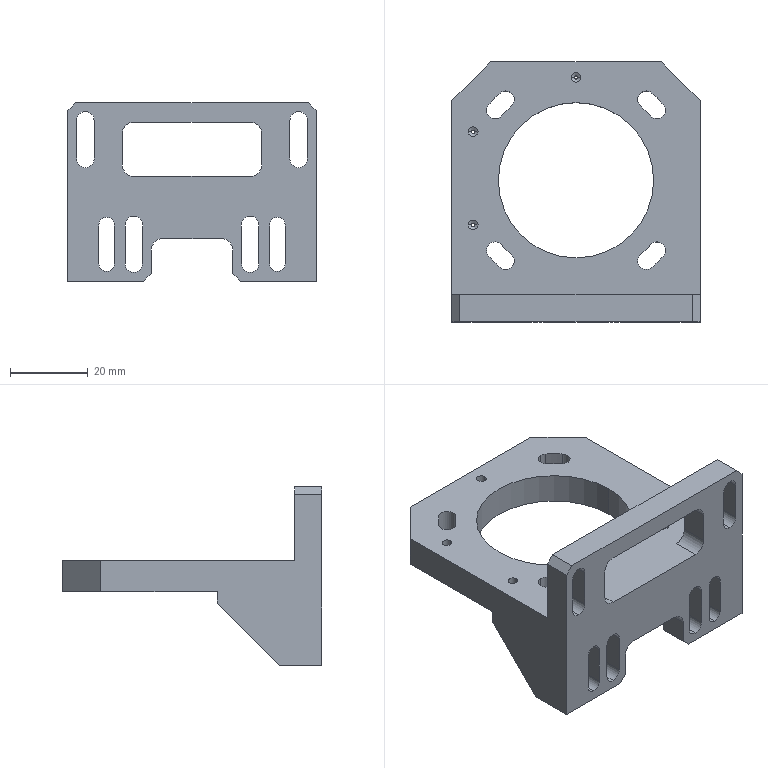NC program | NX | posted with a generic post | part box 64 x 67 x 46 mm
Lines 1 to 1063 of 33790:
N10 G17 G21 G94 G90
(ZLEVEL_PROFILE , TOOL : D10C)
N12 T10 M6
N14 G54
N16 G17 G0 G90 X-38.6 Y9.489 B0. C0. S2500 M3
N18 G43 Z30. H10
N20 Z1.5
N22 G94 G1 Y32.32 Z0.303 F1000.
N24 X-38.483 Y33.131 Z0.261
N26 X-38.238 Y33.914 Z0.218
N28 X-37.871 Y34.647 Z0.175
N30 X-37.392 Y35.312 Z0.132
N32 X-36.812 Y35.892 Z0.089
N34 X-36.147 Y36.371 Z0.046
N36 X-35.414 Y36.738 Z0.003
N38 X-34.631 Y36.983 Z-0.04
N40 X-33.82 Y37.1 Z-0.083
N42 X-33.5 Z-0.1
N44 X23.5 F2500.
N46 G2 X27.106 Y35.606 R5.1
N48 G1 X37.106 Y25.606
N50 G2 X38.6 Y22. R5.1
N52 G1 Y-22.
N54 G2 X37.106 Y-25.606 R5.1
N56 G1 X27.106 Y-35.606
N58 G2 X23.5 Y-37.1 R5.1
N60 G1 X-33.5
N62 G2 X-38.6 Y-32. R5.1
N64 G1 Y32.
N66 G2 X-33.5 Y37.1 R5.1
N68 G1 X-27.771 Z-0.2
N70 X23.5
N72 G2 X27.106 Y35.606 R5.1
N74 G1 X37.106 Y25.606
N76 G2 X38.6 Y22. R5.1
N78 G1 Y-22.
N80 G2 X37.106 Y-25.606 R5.1
N82 G1 X27.106 Y-35.606
N84 G2 X23.5 Y-37.1 R5.1
N86 G1 X-33.5
N88 G2 X-38.6 Y-32. R5.1
N90 G1 Y32.
N92 G2 X-33.5 Y37.1 R5.1
N94 G1 X-27.771 Z-0.3
N96 X23.5
N98 G2 X27.106 Y35.606 R5.1
N100 G1 X37.106 Y25.606
N102 G2 X38.6 Y22. R5.1
N104 G1 Y-22.
N106 G2 X37.106 Y-25.606 R5.1
N108 G1 X27.106 Y-35.606
N110 G2 X23.5 Y-37.1 R5.1
N112 G1 X-33.5
N114 G2 X-38.6 Y-32. R5.1
N116 G1 Y32.
N118 G2 X-33.5 Y37.1 R5.1
N120 G1 X-27.771 Z-0.4
N122 X23.5
N124 G2 X27.106 Y35.606 R5.1
N126 G1 X37.106 Y25.606
N128 G2 X38.6 Y22. R5.1
N130 G1 Y-22.
N132 G2 X37.106 Y-25.606 R5.1
N134 G1 X27.106 Y-35.606
N136 G2 X23.5 Y-37.1 R5.1
N138 G1 X-33.5
N140 G2 X-38.6 Y-32. R5.1
N142 G1 Y32.
N144 G2 X-33.5 Y37.1 R5.1
N146 G1 X-27.771 Z-0.5
N148 X23.5
N150 G2 X27.106 Y35.606 R5.1
N152 G1 X37.106 Y25.606
N154 G2 X38.6 Y22. R5.1
N156 G1 Y-22.
N158 G2 X37.106 Y-25.606 R5.1
N160 G1 X27.106 Y-35.606
N162 G2 X23.5 Y-37.1 R5.1
N164 G1 X-33.5
N166 G2 X-38.6 Y-32. R5.1
N168 G1 Y32.
N170 G2 X-33.5 Y37.1 R5.1
N172 G1 X-27.771 Z-0.6
N174 X23.5
N176 G2 X27.106 Y35.606 R5.1
N178 G1 X37.106 Y25.606
N180 G2 X38.6 Y22. R5.1
N182 G1 Y-22.
N184 G2 X37.106 Y-25.606 R5.1
N186 G1 X27.106 Y-35.606
N188 G2 X23.5 Y-37.1 R5.1
N190 G1 X-33.5
N192 G2 X-38.6 Y-32. R5.1
N194 G1 Y32.
N196 G2 X-33.5 Y37.1 R5.1
N198 G1 X-27.771 Z-0.7
N200 X23.5
N202 G2 X27.106 Y35.606 R5.1
N204 G1 X37.106 Y25.606
N206 G2 X38.6 Y22. R5.1
N208 G1 Y-22.
N210 G2 X37.106 Y-25.606 R5.1
N212 G1 X27.106 Y-35.606
N214 G2 X23.5 Y-37.1 R5.1
N216 G1 X-33.5
N218 G2 X-38.6 Y-32. R5.1
N220 G1 Y32.
N222 G2 X-33.5 Y37.1 R5.1
N224 G1 X-27.771 Z-0.8
N226 X23.5
N228 G2 X27.106 Y35.606 R5.1
N230 G1 X37.106 Y25.606
N232 G2 X38.6 Y22. R5.1
N234 G1 Y-22.
N236 G2 X37.106 Y-25.606 R5.1
N238 G1 X27.106 Y-35.606
N240 G2 X23.5 Y-37.1 R5.1
N242 G1 X-33.5
N244 G2 X-38.6 Y-32. R5.1
N246 G1 Y32.
N248 G2 X-33.5 Y37.1 R5.1
N250 G1 X-27.771 Z-0.9
N252 X23.5
N254 G2 X27.106 Y35.606 R5.1
N256 G1 X37.106 Y25.606
N258 G2 X38.6 Y22. R5.1
N260 G1 Y-22.
N262 G2 X37.106 Y-25.606 R5.1
N264 G1 X27.106 Y-35.606
N266 G2 X23.5 Y-37.1 R5.1
N268 G1 X-33.5
N270 G2 X-38.6 Y-32. R5.1
N272 G1 Y32.
N274 G2 X-33.5 Y37.1 R5.1
N276 G1 X-27.771 Z-1.
N278 X23.5
N280 G2 X27.106 Y35.606 R5.1
N282 G1 X37.106 Y25.606
N284 G2 X38.6 Y22. R5.1
N286 G1 Y-22.
N288 G2 X37.106 Y-25.606 R5.1
N290 G1 X27.106 Y-35.606
N292 G2 X23.5 Y-37.1 R5.1
N294 G1 X-33.5
N296 G2 X-38.6 Y-32. R5.1
N298 G1 Y32.
N300 G2 X-33.5 Y37.1 R5.1
N302 G1 X-27.771 Z-1.1
N304 X23.5
N306 G2 X27.106 Y35.606 R5.1
N308 G1 X37.106 Y25.606
N310 G2 X38.6 Y22. R5.1
N312 G1 Y-22.
N314 G2 X37.106 Y-25.606 R5.1
N316 G1 X27.106 Y-35.606
N318 G2 X23.5 Y-37.1 R5.1
N320 G1 X-33.5
N322 G2 X-38.6 Y-32. R5.1
N324 G1 Y32.
N326 G2 X-33.5 Y37.1 R5.1
N328 G1 X-27.771 Z-1.2
N330 X23.5
N332 G2 X27.106 Y35.606 R5.1
N334 G1 X37.106 Y25.606
N336 G2 X38.6 Y22. R5.1
N338 G1 Y-22.
N340 G2 X37.106 Y-25.606 R5.1
N342 G1 X27.106 Y-35.606
N344 G2 X23.5 Y-37.1 R5.1
N346 G1 X-33.5
N348 G2 X-38.6 Y-32. R5.1
N350 G1 Y32.
N352 G2 X-33.5 Y37.1 R5.1
N354 G1 X-27.771 Z-1.3
N356 X23.5
N358 G2 X27.106 Y35.606 R5.1
N360 G1 X37.106 Y25.606
N362 G2 X38.6 Y22. R5.1
N364 G1 Y-22.
N366 G2 X37.106 Y-25.606 R5.1
N368 G1 X27.106 Y-35.606
N370 G2 X23.5 Y-37.1 R5.1
N372 G1 X-33.5
N374 G2 X-38.6 Y-32. R5.1
N376 G1 Y32.
N378 G2 X-33.5 Y37.1 R5.1
N380 G1 X-27.771 Z-1.4
N382 X23.5
N384 G2 X27.106 Y35.606 R5.1
N386 G1 X37.106 Y25.606
N388 G2 X38.6 Y22. R5.1
N390 G1 Y-22.
N392 G2 X37.106 Y-25.606 R5.1
N394 G1 X27.106 Y-35.606
N396 G2 X23.5 Y-37.1 R5.1
N398 G1 X-33.5
N400 G2 X-38.6 Y-32. R5.1
N402 G1 Y32.
N404 G2 X-33.5 Y37.1 R5.1
N406 G1 X-27.771 Z-1.5
N408 X23.5
N410 G2 X27.106 Y35.606 R5.1
N412 G1 X37.106 Y25.606
N414 G2 X38.6 Y22. R5.1
N416 G1 Y-22.
N418 G2 X37.106 Y-25.606 R5.1
N420 G1 X27.106 Y-35.606
N422 G2 X23.5 Y-37.1 R5.1
N424 G1 X-33.5
N426 G2 X-38.6 Y-32. R5.1
N428 G1 Y32.
N430 G2 X-33.5 Y37.1 R5.1
N432 G1 X-27.771 Z-1.6
N434 X23.5
N436 G2 X27.106 Y35.606 R5.1
N438 G1 X37.106 Y25.606
N440 G2 X38.6 Y22. R5.1
N442 G1 Y-22.
N444 G2 X37.106 Y-25.606 R5.1
N446 G1 X27.106 Y-35.606
N448 G2 X23.5 Y-37.1 R5.1
N450 G1 X-33.5
N452 G2 X-38.6 Y-32. R5.1
N454 G1 Y32.
N456 G2 X-33.5 Y37.1 R5.1
N458 G1 X-27.771 Z-1.7
N460 X23.5
N462 G2 X27.106 Y35.606 R5.1
N464 G1 X37.106 Y25.606
N466 G2 X38.6 Y22. R5.1
N468 G1 Y-22.
N470 G2 X37.106 Y-25.606 R5.1
N472 G1 X27.106 Y-35.606
N474 G2 X23.5 Y-37.1 R5.1
N476 G1 X-33.5
N478 G2 X-38.6 Y-32. R5.1
N480 G1 Y32.
N482 G2 X-33.5 Y37.1 R5.1
N484 G1 X-27.771 Z-1.8
N486 X23.5
N488 G2 X27.106 Y35.606 R5.1
N490 G1 X37.106 Y25.606
N492 G2 X38.6 Y22. R5.1
N494 G1 Y-22.
N496 G2 X37.106 Y-25.606 R5.1
N498 G1 X27.106 Y-35.606
N500 G2 X23.5 Y-37.1 R5.1
N502 G1 X-33.5
N504 G2 X-38.6 Y-32. R5.1
N506 G1 Y32.
N508 G2 X-33.5 Y37.1 R5.1
N510 G1 X-27.771 Z-1.9
N512 X23.5
N514 G2 X27.106 Y35.606 R5.1
N516 G1 X37.106 Y25.606
N518 G2 X38.6 Y22. R5.1
N520 G1 Y-22.
N522 G2 X37.106 Y-25.606 R5.1
N524 G1 X27.106 Y-35.606
N526 G2 X23.5 Y-37.1 R5.1
N528 G1 X-33.5
N530 G2 X-38.6 Y-32. R5.1
N532 G1 Y32.
N534 G2 X-33.5 Y37.1 R5.1
N536 G1 X-27.771 Z-2.
N538 X23.5
N540 G2 X27.106 Y35.606 R5.1
N542 G1 X37.106 Y25.606
N544 G2 X38.6 Y22. R5.1
N546 G1 Y-22.
N548 G2 X37.106 Y-25.606 R5.1
N550 G1 X27.106 Y-35.606
N552 G2 X23.5 Y-37.1 R5.1
N554 G1 X-33.5
N556 G2 X-38.6 Y-32. R5.1
N558 G1 Y32.
N560 G2 X-33.5 Y37.1 R5.1
N562 G1 X-27.771 Z-2.1
N564 X23.5
N566 G2 X27.106 Y35.606 R5.1
N568 G1 X37.106 Y25.606
N570 G2 X38.6 Y22. R5.1
N572 G1 Y-22.
N574 G2 X37.106 Y-25.606 R5.1
N576 G1 X27.106 Y-35.606
N578 G2 X23.5 Y-37.1 R5.1
N580 G1 X-33.5
N582 G2 X-38.6 Y-32. R5.1
N584 G1 Y32.
N586 G2 X-33.5 Y37.1 R5.1
N588 G1 X-27.771 Z-2.2
N590 X23.5
N592 G2 X27.106 Y35.606 R5.1
N594 G1 X37.106 Y25.606
N596 G2 X38.6 Y22. R5.1
N598 G1 Y-22.
N600 G2 X37.106 Y-25.606 R5.1
N602 G1 X27.106 Y-35.606
N604 G2 X23.5 Y-37.1 R5.1
N606 G1 X-33.5
N608 G2 X-38.6 Y-32. R5.1
N610 G1 Y32.
N612 G2 X-33.5 Y37.1 R5.1
N614 G1 X-27.771 Z-2.3
N616 X23.5
N618 G2 X27.106 Y35.606 R5.1
N620 G1 X37.106 Y25.606
N622 G2 X38.6 Y22. R5.1
N624 G1 Y-22.
N626 G2 X37.106 Y-25.606 R5.1
N628 G1 X27.106 Y-35.606
N630 G2 X23.5 Y-37.1 R5.1
N632 G1 X-33.5
N634 G2 X-38.6 Y-32. R5.1
N636 G1 Y32.
N638 G2 X-33.5 Y37.1 R5.1
N640 G1 X-27.771 Z-2.4
N642 X23.5
N644 G2 X27.106 Y35.606 R5.1
N646 G1 X37.106 Y25.606
N648 G2 X38.6 Y22. R5.1
N650 G1 Y-22.
N652 G2 X37.106 Y-25.606 R5.1
N654 G1 X27.106 Y-35.606
N656 G2 X23.5 Y-37.1 R5.1
N658 G1 X-33.5
N660 G2 X-38.6 Y-32. R5.1
N662 G1 Y32.
N664 G2 X-33.5 Y37.1 R5.1
N666 G1 X-27.771 Z-2.5
N668 X23.5
N670 G2 X27.106 Y35.606 R5.1
N672 G1 X37.106 Y25.606
N674 G2 X38.6 Y22. R5.1
N676 G1 Y-22.
N678 G2 X37.106 Y-25.606 R5.1
N680 G1 X27.106 Y-35.606
N682 G2 X23.5 Y-37.1 R5.1
N684 G1 X-33.5
N686 G2 X-38.6 Y-32. R5.1
N688 G1 Y32.
N690 G2 X-33.5 Y37.1 R5.1
N692 G1 X-27.771 Z-2.6
N694 X23.5
N696 G2 X27.106 Y35.606 R5.1
N698 G1 X37.106 Y25.606
N700 G2 X38.6 Y22. R5.1
N702 G1 Y-22.
N704 G2 X37.106 Y-25.606 R5.1
N706 G1 X27.106 Y-35.606
N708 G2 X23.5 Y-37.1 R5.1
N710 G1 X-33.5
N712 G2 X-38.6 Y-32. R5.1
N714 G1 Y32.
N716 G2 X-33.5 Y37.1 R5.1
N718 G1 X-27.771 Z-2.7
N720 X23.5
N722 G2 X27.106 Y35.606 R5.1
N724 G1 X37.106 Y25.606
N726 G2 X38.6 Y22. R5.1
N728 G1 Y-22.
N730 G2 X37.106 Y-25.606 R5.1
N732 G1 X27.106 Y-35.606
N734 G2 X23.5 Y-37.1 R5.1
N736 G1 X-33.5
N738 G2 X-38.6 Y-32. R5.1
N740 G1 Y32.
N742 G2 X-33.5 Y37.1 R5.1
N744 G1 X-27.771 Z-2.8
N746 X23.5
N748 G2 X27.106 Y35.606 R5.1
N750 G1 X37.106 Y25.606
N752 G2 X38.6 Y22. R5.1
N754 G1 Y-22.
N756 G2 X37.106 Y-25.606 R5.1
N758 G1 X27.106 Y-35.606
N760 G2 X23.5 Y-37.1 R5.1
N762 G1 X-33.5
N764 G2 X-38.6 Y-32. R5.1
N766 G1 Y32.
N768 G2 X-33.5 Y37.1 R5.1
N770 G1 X-27.771 Z-2.9
N772 X23.5
N774 G2 X27.106 Y35.606 R5.1
N776 G1 X37.106 Y25.606
N778 G2 X38.6 Y22. R5.1
N780 G1 Y-22.
N782 G2 X37.106 Y-25.606 R5.1
N784 G1 X27.106 Y-35.606
N786 G2 X23.5 Y-37.1 R5.1
N788 G1 X-33.5
N790 G2 X-38.6 Y-32. R5.1
N792 G1 Y32.
N794 G2 X-33.5 Y37.1 R5.1
N796 G1 X-27.771 Z-3.
N798 X23.5
N800 G2 X27.106 Y35.606 R5.1
N802 G1 X37.106 Y25.606
N804 G2 X38.6 Y22. R5.1
N806 G1 Y-22.
N808 G2 X37.106 Y-25.606 R5.1
N810 G1 X27.106 Y-35.606
N812 G2 X23.5 Y-37.1 R5.1
N814 G1 X-33.5
N816 G2 X-38.6 Y-32. R5.1
N818 G1 Y32.
N820 G2 X-33.5 Y37.1 R5.1
N822 G1 X-27.771 Z-3.1
N824 X23.5
N826 G2 X27.106 Y35.606 R5.1
N828 G1 X37.106 Y25.606
N830 G2 X38.6 Y22. R5.1
N832 G1 Y-22.
N834 G2 X37.106 Y-25.606 R5.1
N836 G1 X27.106 Y-35.606
N838 G2 X23.5 Y-37.1 R5.1
N840 G1 X-33.5
N842 G2 X-38.6 Y-32. R5.1
N844 G1 Y32.
N846 G2 X-33.5 Y37.1 R5.1
N848 G1 X-27.771 Z-3.2
N850 X23.5
N852 G2 X27.106 Y35.606 R5.1
N854 G1 X37.106 Y25.606
N856 G2 X38.6 Y22. R5.1
N858 G1 Y-22.
N860 G2 X37.106 Y-25.606 R5.1
N862 G1 X27.106 Y-35.606
N864 G2 X23.5 Y-37.1 R5.1
N866 G1 X-33.5
N868 G2 X-38.6 Y-32. R5.1
N870 G1 Y32.
N872 G2 X-33.5 Y37.1 R5.1
N874 G1 X-27.771 Z-3.3
N876 X23.5
N878 G2 X27.106 Y35.606 R5.1
N880 G1 X37.106 Y25.606
N882 G2 X38.6 Y22. R5.1
N884 G1 Y-22.
N886 G2 X37.106 Y-25.606 R5.1
N888 G1 X27.106 Y-35.606
N890 G2 X23.5 Y-37.1 R5.1
N892 G1 X-33.5
N894 G2 X-38.6 Y-32. R5.1
N896 G1 Y32.
N898 G2 X-33.5 Y37.1 R5.1
N900 G1 X-27.771 Z-3.4
N902 X23.5
N904 G2 X27.106 Y35.606 R5.1
N906 G1 X37.106 Y25.606
N908 G2 X38.6 Y22. R5.1
N910 G1 Y-22.
N912 G2 X37.106 Y-25.606 R5.1
N914 G1 X27.106 Y-35.606
N916 G2 X23.5 Y-37.1 R5.1
N918 G1 X-33.5
N920 G2 X-38.6 Y-32. R5.1
N922 G1 Y32.
N924 G2 X-33.5 Y37.1 R5.1
N926 G1 X-27.771 Z-3.5
N928 X23.5
N930 G2 X27.106 Y35.606 R5.1
N932 G1 X37.106 Y25.606
N934 G2 X38.6 Y22. R5.1
N936 G1 Y-22.
N938 G2 X37.106 Y-25.606 R5.1
N940 G1 X27.106 Y-35.606
N942 G2 X23.5 Y-37.1 R5.1
N944 G1 X-33.5
N946 G2 X-38.6 Y-32. R5.1
N948 G1 Y32.
N950 G2 X-33.5 Y37.1 R5.1
N952 G1 X-27.771 Z-3.6
N954 X23.5
N956 G2 X27.106 Y35.606 R5.1
N958 G1 X37.106 Y25.606
N960 G2 X38.6 Y22. R5.1
N962 G1 Y-22.
N964 G2 X37.106 Y-25.606 R5.1
N966 G1 X27.106 Y-35.606
N968 G2 X23.5 Y-37.1 R5.1
N970 G1 X-33.5
N972 G2 X-38.6 Y-32. R5.1
N974 G1 Y32.
N976 G2 X-33.5 Y37.1 R5.1
N978 G1 X-27.771 Z-3.7
N980 X23.5
N982 G2 X27.106 Y35.606 R5.1
N984 G1 X37.106 Y25.606
N986 G2 X38.6 Y22. R5.1
N988 G1 Y-22.
N990 G2 X37.106 Y-25.606 R5.1
N992 G1 X27.106 Y-35.606
N994 G2 X23.5 Y-37.1 R5.1
N996 G1 X-33.5
N998 G2 X-38.6 Y-32. R5.1
N1000 G1 Y32.
N1002 G2 X-33.5 Y37.1 R5.1
N1004 G1 X-27.771 Z-3.8
N1006 X23.5
N1008 G2 X27.106 Y35.606 R5.1
N1010 G1 X37.106 Y25.606
N1012 G2 X38.6 Y22. R5.1
N1014 G1 Y-22.
N1016 G2 X37.106 Y-25.606 R5.1
N1018 G1 X27.106 Y-35.606
N1020 G2 X23.5 Y-37.1 R5.1
N1022 G1 X-33.5
N1024 G2 X-38.6 Y-32. R5.1
N1026 G1 Y32.
N1028 G2 X-33.5 Y37.1 R5.1
N1030 G1 X-27.771 Z-3.9
N1032 X23.5
N1034 G2 X27.106 Y35.606 R5.1
N1036 G1 X37.106 Y25.606
N1038 G2 X38.6 Y22. R5.1
N1040 G1 Y-22.
N1042 G2 X37.106 Y-25.606 R5.1
N1044 G1 X27.106 Y-35.606
N1046 G2 X23.5 Y-37.1 R5.1
N1048 G1 X-33.5
N1050 G2 X-38.6 Y-32. R5.1
N1052 G1 Y32.
N1054 G2 X-33.5 Y37.1 R5.1
N1056 G1 X-27.771 Z-4.
N1058 X23.5
N1060 G2 X27.106 Y35.606 R5.1
N1062 G1 X37.106 Y25.606
N1064 G2 X38.6 Y22. R5.1
N1066 G1 Y-22.
N1068 G2 X37.106 Y-25.606 R5.1
N1070 G1 X27.106 Y-35.606
N1072 G2 X23.5 Y-37.1 R5.1
N1074 G1 X-33.5
N1076 G2 X-38.6 Y-32. R5.1
N1078 G1 Y32.
N1080 G2 X-33.5 Y37.1 R5.1
N1082 G1 X-27.771 Z-4.1
N1084 X23.5
N1086 G2 X27.106 Y35.606 R5.1
N1088 G1 X37.106 Y25.606
N1090 G2 X38.6 Y22. R5.1
N1092 G1 Y-22.
N1094 G2 X37.106 Y-25.606 R5.1
N1096 G1 X27.106 Y-35.606
N1098 G2 X23.5 Y-37.1 R5.1
N1100 G1 X-33.5
N1102 G2 X-38.6 Y-32. R5.1
N1104 G1 Y32.
N1106 G2 X-33.5 Y37.1 R5.1
N1108 G1 X-27.771 Z-4.2
N1110 X23.5
N1112 G2 X27.106 Y35.606 R5.1
N1114 G1 X37.106 Y25.606
N1116 G2 X38.6 Y22. R5.1
N1118 G1 Y-22.
N1120 G2 X37.106 Y-25.606 R5.1
N1122 G1 X27.106 Y-35.606
N1124 G2 X23.5 Y-37.1 R5.1
N1126 G1 X-33.5
N1128 G2 X-38.6 Y-32. R5.1
N1130 G1 Y32.
N1132 G2 X-33.5 Y37.1 R5.1
N1134 G1 X-27.771 Z-4.3
N1136 X23.5
N1138 G2 X27.106 Y35.606 R5.1
N1140 G1 X37.106 Y25.606
N1142 G2 X38.6 Y22. R5.1
N1144 G1 Y-22.
N1146 G2 X37.106 Y-25.606 R5.1
N1148 G1 X27.106 Y-35.606
N1150 G2 X23.5 Y-37.1 R5.1
N1152 G1 X-33.5
N1154 G2 X-38.6 Y-32. R5.1
N1156 G1 Y32.
N1158 G2 X-33.5 Y37.1 R5.1
N1160 G1 X-27.771 Z-4.4
N1162 X23.5
N1164 G2 X27.106 Y35.606 R5.1
N1166 G1 X37.106 Y25.606
N1168 G2 X38.6 Y22. R5.1
N1170 G1 Y-22.
N1172 G2 X37.106 Y-25.606 R5.1
N1174 G1 X27.106 Y-35.606
N1176 G2 X23.5 Y-37.1 R5.1
N1178 G1 X-33.5
N1180 G2 X-38.6 Y-32. R5.1
N1182 G1 Y32.
N1184 G2 X-33.5 Y37.1 R5.1
N1186 G1 X-27.771 Z-4.5
N1188 X23.5
N1190 G2 X27.106 Y35.606 R5.1
N1192 G1 X37.106 Y25.606
N1194 G2 X38.6 Y22. R5.1
N1196 G1 Y-22.
N1198 G2 X37.106 Y-25.606 R5.1
N1200 G1 X27.106 Y-35.606
N1202 G2 X23.5 Y-37.1 R5.1
N1204 G1 X-33.5
N1206 G2 X-38.6 Y-32. R5.1
N1208 G1 Y32.
N1210 G2 X-33.5 Y37.1 R5.1
N1212 G1 X-27.771 Z-4.6
N1214 X23.5
N1216 G2 X27.106 Y35.606 R5.1
N1218 G1 X37.106 Y25.606
N1220 G2 X38.6 Y22. R5.1
N1222 G1 Y-22.
N1224 G2 X37.106 Y-25.606 R5.1
N1226 G1 X27.106 Y-35.606
N1228 G2 X23.5 Y-37.1 R5.1
N1230 G1 X-33.5
N1232 G2 X-38.6 Y-32. R5.1
N1234 G1 Y32.
N1236 G2 X-33.5 Y37.1 R5.1
N1238 G1 X-27.771 Z-4.7
N1240 X23.5
N1242 G2 X27.106 Y35.606 R5.1
N1244 G1 X37.106 Y25.606
N1246 G2 X38.6 Y22. R5.1
N1248 G1 Y-22.
N1250 G2 X37.106 Y-25.606 R5.1
N1252 G1 X27.106 Y-35.606
N1254 G2 X23.5 Y-37.1 R5.1
N1256 G1 X-33.5
N1258 G2 X-38.6 Y-32. R5.1
N1260 G1 Y32.
N1262 G2 X-33.5 Y37.1 R5.1
N1264 G1 X-27.771 Z-4.8
N1266 X23.5
N1268 G2 X27.106 Y35.606 R5.1
N1270 G1 X37.106 Y25.606
N1272 G2 X38.6 Y22. R5.1
N1274 G1 Y-22.
N1276 G2 X37.106 Y-25.606 R5.1
N1278 G1 X27.106 Y-35.606
N1280 G2 X23.5 Y-37.1 R5.1
N1282 G1 X-33.5
N1284 G2 X-38.6 Y-32. R5.1
N1286 G1 Y32.
N1288 G2 X-33.5 Y37.1 R5.1
N1290 G1 X-27.771 Z-4.9
N1292 X23.5
N1294 G2 X27.106 Y35.606 R5.1
N1296 G1 X37.106 Y25.606
N1298 G2 X38.6 Y22. R5.1
N1300 G1 Y-22.
N1302 G2 X37.106 Y-25.606 R5.1
N1304 G1 X27.106 Y-35.606
N1306 G2 X23.5 Y-37.1 R5.1
N1308 G1 X-33.5
N1310 G2 X-38.6 Y-32. R5.1
N1312 G1 Y32.
N1314 G2 X-33.5 Y37.1 R5.1
N1316 G1 X-27.771 Z-5.
N1318 X23.5
N1320 G2 X27.106 Y35.606 R5.1
N1322 G1 X37.106 Y25.606
N1324 G2 X38.6 Y22. R5.1
N1326 G1 Y-22.
N1328 G2 X37.106 Y-25.606 R5.1
N1330 G1 X27.106 Y-35.606
N1332 G2 X23.5 Y-37.1 R5.1
N1334 G1 X-33.5
N1336 G2 X-38.6 Y-32. R5.1
N1338 G1 Y32.
N1340 G2 X-33.5 Y37.1 R5.1
N1342 G1 X-27.771 Z-5.1
N1344 X23.5
N1346 G2 X27.106 Y35.606 R5.1
N1348 G1 X37.106 Y25.606
N1350 G2 X38.6 Y22. R5.1
N1352 G1 Y-22.
N1354 G2 X37.106 Y-25.606 R5.1
N1356 G1 X27.106 Y-35.606
N1358 G2 X23.5 Y-37.1 R5.1
N1360 G1 X-33.5
N1362 G2 X-38.6 Y-32. R5.1
N1364 G1 Y32.
N1366 G2 X-33.5 Y37.1 R5.1
N1368 G1 X-27.771 Z-5.2
N1370 X23.5
N1372 G2 X27.106 Y35.606 R5.1
N1374 G1 X37.106 Y25.606
N1376 G2 X38.6 Y22. R5.1
N1378 G1 Y-22.
N1380 G2 X37.106 Y-25.606 R5.1
N1382 G1 X27.106 Y-35.606
N1384 G2 X23.5 Y-37.1 R5.1
N1386 G1 X-33.5
N1388 G2 X-38.6 Y-32. R5.1
N1390 G1 Y32.
N1392 G2 X-33.5 Y37.1 R5.1
N1394 G1 X-27.771 Z-5.3
N1396 X23.5
N1398 G2 X27.106 Y35.606 R5.1
N1400 G1 X37.106 Y25.606
N1402 G2 X38.6 Y22. R5.1
N1404 G1 Y-22.
N1406 G2 X37.106 Y-25.606 R5.1
N1408 G1 X27.106 Y-35.606
N1410 G2 X23.5 Y-37.1 R5.1
N1412 G1 X-33.5
N1414 G2 X-38.6 Y-32. R5.1
N1416 G1 Y32.
N1418 G2 X-33.5 Y37.1 R5.1
N1420 G1 X-27.771 Z-5.4
N1422 X23.5
N1424 G2 X27.106 Y35.606 R5.1
N1426 G1 X37.106 Y25.606
N1428 G2 X38.6 Y22. R5.1
N1430 G1 Y-22.
N1432 G2 X37.106 Y-25.606 R5.1
N1434 G1 X27.106 Y-35.606
N1436 G2 X23.5 Y-37.1 R5.1
N1438 G1 X-33.5
N1440 G2 X-38.6 Y-32. R5.1
N1442 G1 Y32.
N1444 G2 X-33.5 Y37.1 R5.1
N1446 G1 X-27.771 Z-5.5
N1448 X23.5
N1450 G2 X27.106 Y35.606 R5.1
N1452 G1 X37.106 Y25.606
N1454 G2 X38.6 Y22. R5.1
N1456 G1 Y-22.
N1458 G2 X37.106 Y-25.606 R5.1
N1460 G1 X27.106 Y-35.606
N1462 G2 X23.5 Y-37.1 R5.1
N1464 G1 X-33.5
N1466 G2 X-38.6 Y-32. R5.1
N1468 G1 Y32.
N1470 G2 X-33.5 Y37.1 R5.1
N1472 G1 X-27.771 Z-5.6
N1474 X23.5
N1476 G2 X27.106 Y35.606 R5.1
N1478 G1 X37.106 Y25.606
N1480 G2 X38.6 Y22. R5.1
N1482 G1 Y-22.
N1484 G2 X37.106 Y-25.606 R5.1
N1486 G1 X27.106 Y-35.606
N1488 G2 X23.5 Y-37.1 R5.1
N1490 G1 X-33.5
N1492 G2 X-38.6 Y-32. R5.1
N1494 G1 Y32.
N1496 G2 X-33.5 Y37.1 R5.1
N1498 G1 X-27.771 Z-5.7
N1500 X23.5
N1502 G2 X27.106 Y35.606 R5.1
N1504 G1 X37.106 Y25.606
N1506 G2 X38.6 Y22. R5.1
N1508 G1 Y-22.
N1510 G2 X37.106 Y-25.606 R5.1
N1512 G1 X27.106 Y-35.606
N1514 G2 X23.5 Y-37.1 R5.1
N1516 G1 X-33.5
N1518 G2 X-38.6 Y-32. R5.1
N1520 G1 Y32.
N1522 G2 X-33.5 Y37.1 R5.1
N1524 G1 X-27.771 Z-5.8
N1526 X23.5
N1528 G2 X27.106 Y35.606 R5.1
N1530 G1 X37.106 Y25.606
N1532 G2 X38.6 Y22. R5.1
N1534 G1 Y-22.
N1536 G2 X37.106 Y-25.606 R5.1
N1538 G1 X27.106 Y-35.606
N1540 G2 X23.5 Y-37.1 R5.1
N1542 G1 X-33.5
N1544 G2 X-38.6 Y-32. R5.1
N1546 G1 Y32.
N1548 G2 X-33.5 Y37.1 R5.1
N1550 G1 X-27.771 Z-5.9
N1552 X23.5
N1554 G2 X27.106 Y35.606 R5.1
N1556 G1 X37.106 Y25.606
N1558 G2 X38.6 Y22. R5.1
N1560 G1 Y-22.
N1562 G2 X37.106 Y-25.606 R5.1
N1564 G1 X27.106 Y-35.606
N1566 G2 X23.5 Y-37.1 R5.1
N1568 G1 X-33.5
N1570 G2 X-38.6 Y-32. R5.1
N1572 G1 Y32.
N1574 G2 X-33.5 Y37.1 R5.1
N1576 G1 X-27.771 Z-6.
N1578 X23.5
N1580 G2 X27.106 Y35.606 R5.1
N1582 G1 X37.106 Y25.606
N1584 G2 X38.6 Y22. R5.1
N1586 G1 Y-22.
N1588 G2 X37.106 Y-25.606 R5.1
N1590 G1 X27.106 Y-35.606
N1592 G2 X23.5 Y-37.1 R5.1
N1594 G1 X-33.5
N1596 G2 X-38.6 Y-32. R5.1
N1598 G1 Y32.
N1600 G2 X-33.5 Y37.1 R5.1
N1602 G1 X-27.771 Z-6.1
N1604 X23.5
N1606 G2 X27.106 Y35.606 R5.1
N1608 G1 X37.106 Y25.606
N1610 G2 X38.6 Y22. R5.1
N1612 G1 Y-22.
N1614 G2 X37.106 Y-25.606 R5.1
N1616 G1 X27.106 Y-35.606
N1618 G2 X23.5 Y-37.1 R5.1
N1620 G1 X-33.5
N1622 G2 X-38.6 Y-32. R5.1
N1624 G1 Y32.
N1626 G2 X-33.5 Y37.1 R5.1
N1628 G1 X-27.771 Z-6.2
N1630 X23.5
N1632 G2 X27.106 Y35.606 R5.1
N1634 G1 X37.106 Y25.606
N1636 G2 X38.6 Y22. R5.1
N1638 G1 Y-22.
N1640 G2 X37.106 Y-25.606 R5.1
N1642 G1 X27.106 Y-35.606
N1644 G2 X23.5 Y-37.1 R5.1
N1646 G1 X-33.5
N1648 G2 X-38.6 Y-32. R5.1
N1650 G1 Y32.
N1652 G2 X-33.5 Y37.1 R5.1
N1654 G1 X-27.771 Z-6.3
N1656 X23.5
N1658 G2 X27.106 Y35.606 R5.1
N1660 G1 X37.106 Y25.606
N1662 G2 X38.6 Y22. R5.1
N1664 G1 Y-22.
N1666 G2 X37.106 Y-25.606 R5.1
N1668 G1 X27.106 Y-35.606
N1670 G2 X23.5 Y-37.1 R5.1
N1672 G1 X-33.5
N1674 G2 X-38.6 Y-32. R5.1
N1676 G1 Y32.
N1678 G2 X-33.5 Y37.1 R5.1
N1680 G1 X-27.771 Z-6.4
N1682 X23.5
N1684 G2 X27.106 Y35.606 R5.1
N1686 G1 X37.106 Y25.606
N1688 G2 X38.6 Y22. R5.1
N1690 G1 Y-22.
N1692 G2 X37.106 Y-25.606 R5.1
N1694 G1 X27.106 Y-35.606
N1696 G2 X23.5 Y-37.1 R5.1
N1698 G1 X-33.5
N1700 G2 X-38.6 Y-32. R5.1
N1702 G1 Y32.
N1704 G2 X-33.5 Y37.1 R5.1
N1706 G1 X-27.771 Z-6.5
N1708 X23.5
N1710 G2 X27.106 Y35.606 R5.1
N1712 G1 X37.106 Y25.606
N1714 G2 X38.6 Y22. R5.1
N1716 G1 Y-22.
N1718 G2 X37.106 Y-25.606 R5.1
N1720 G1 X27.106 Y-35.606
N1722 G2 X23.5 Y-37.1 R5.1
N1724 G1 X-33.5
N1726 G2 X-38.6 Y-32. R5.1
N1728 G1 Y32.
N1730 G2 X-33.5 Y37.1 R5.1
N1732 G1 X-27.771 Z-6.6
N1734 X23.5
N1736 G2 X27.106 Y35.606 R5.1
N1738 G1 X37.106 Y25.606
N1740 G2 X38.6 Y22. R5.1
N1742 G1 Y-22.
N1744 G2 X37.106 Y-25.606 R5.1
N1746 G1 X27.106 Y-35.606
N1748 G2 X23.5 Y-37.1 R5.1
N1750 G1 X-33.5
N1752 G2 X-38.6 Y-32. R5.1
N1754 G1 Y32.
N1756 G2 X-33.5 Y37.1 R5.1
N1758 G1 X-27.771 Z-6.7
N1760 X23.5
N1762 G2 X27.106 Y35.606 R5.1
N1764 G1 X37.106 Y25.606
N1766 G2 X38.6 Y22. R5.1
N1768 G1 Y-22.
N1770 G2 X37.106 Y-25.606 R5.1
N1772 G1 X27.106 Y-35.606
N1774 G2 X23.5 Y-37.1 R5.1
N1776 G1 X-33.5
N1778 G2 X-38.6 Y-32. R5.1
N1780 G1 Y32.
N1782 G2 X-33.5 Y37.1 R5.1
N1784 G1 X-27.771 Z-6.8
N1786 X23.5
N1788 G2 X27.106 Y35.606 R5.1
N1790 G1 X37.106 Y25.606
N1792 G2 X38.6 Y22. R5.1
N1794 G1 Y-22.
N1796 G2 X37.106 Y-25.606 R5.1
N1798 G1 X27.106 Y-35.606
N1800 G2 X23.5 Y-37.1 R5.1
N1802 G1 X-33.5
N1804 G2 X-38.6 Y-32. R5.1
N1806 G1 Y32.
N1808 G2 X-33.5 Y37.1 R5.1
N1810 G1 X-27.771 Z-6.9
N1812 X23.5
N1814 G2 X27.106 Y35.606 R5.1
N1816 G1 X37.106 Y25.606
N1818 G2 X38.6 Y22. R5.1
N1820 G1 Y-22.
N1822 G2 X37.106 Y-25.606 R5.1
N1824 G1 X27.106 Y-35.606
N1826 G2 X23.5 Y-37.1 R5.1
N1828 G1 X-33.5
N1830 G2 X-38.6 Y-32. R5.1
N1832 G1 Y32.
N1834 G2 X-33.5 Y37.1 R5.1
N1836 G1 X-27.771 Z-7.
N1838 X23.5
N1840 G2 X27.106 Y35.606 R5.1
N1842 G1 X37.106 Y25.606
N1844 G2 X38.6 Y22. R5.1
N1846 G1 Y-22.
N1848 G2 X37.106 Y-25.606 R5.1
N1850 G1 X27.106 Y-35.606
N1852 G2 X23.5 Y-37.1 R5.1
N1854 G1 X-33.5
N1856 G2 X-38.6 Y-32. R5.1
N1858 G1 Y32.
N1860 G2 X-33.5 Y37.1 R5.1
N1862 G1 X-27.771 Z-7.1
N1864 X23.5
N1866 G2 X27.106 Y35.606 R5.1
N1868 G1 X37.106 Y25.606
N1870 G2 X38.6 Y22. R5.1
N1872 G1 Y-22.
N1874 G2 X37.106 Y-25.606 R5.1
N1876 G1 X27.106 Y-35.606
N1878 G2 X23.5 Y-37.1 R5.1
N1880 G1 X-33.5
N1882 G2 X-38.6 Y-32. R5.1
N1884 G1 Y32.
N1886 G2 X-33.5 Y37.1 R5.1
N1888 G1 X-27.771 Z-7.2
N1890 X23.5
N1892 G2 X27.106 Y35.606 R5.1
N1894 G1 X37.106 Y25.606
N1896 G2 X38.6 Y22. R5.1
N1898 G1 Y-22.
N1900 G2 X37.106 Y-25.606 R5.1
N1902 G1 X27.106 Y-35.606
N1904 G2 X23.5 Y-37.1 R5.1
N1906 G1 X-33.5
N1908 G2 X-38.6 Y-32. R5.1
N1910 G1 Y32.
N1912 G2 X-33.5 Y37.1 R5.1
N1914 G1 X-27.771 Z-7.3
N1916 X23.5
N1918 G2 X27.106 Y35.606 R5.1
N1920 G1 X37.106 Y25.606
N1922 G2 X38.6 Y22. R5.1
N1924 G1 Y-22.
N1926 G2 X37.106 Y-25.606 R5.1
N1928 G1 X27.106 Y-35.606
N1930 G2 X23.5 Y-37.1 R5.1
N1932 G1 X-33.5
N1934 G2 X-38.6 Y-32. R5.1
N1936 G1 Y32.
N1938 G2 X-33.5 Y37.1 R5.1
N1940 G1 X-27.771 Z-7.4
N1942 X23.5
N1944 G2 X27.106 Y35.606 R5.1
N1946 G1 X37.106 Y25.606
N1948 G2 X38.6 Y22. R5.1
N1950 G1 Y-22.
N1952 G2 X37.106 Y-25.606 R5.1
N1954 G1 X27.106 Y-35.606
N1956 G2 X23.5 Y-37.1 R5.1
N1958 G1 X-33.5
N1960 G2 X-38.6 Y-32. R5.1
N1962 G1 Y32.
N1964 G2 X-33.5 Y37.1 R5.1
N1966 G1 X-27.771 Z-7.5
N1968 X23.5
N1970 G2 X27.106 Y35.606 R5.1
N1972 G1 X37.106 Y25.606
N1974 G2 X38.6 Y22. R5.1
N1976 G1 Y-22.
N1978 G2 X37.106 Y-25.606 R5.1
N1980 G1 X27.106 Y-35.606
N1982 G2 X23.5 Y-37.1 R5.1
N1984 G1 X-33.5
N1986 G2 X-38.6 Y-32. R5.1
N1988 G1 Y32.
N1990 G2 X-33.5 Y37.1 R5.1
N1992 G1 X-27.771 Z-7.6
N1994 X23.5
N1996 G2 X27.106 Y35.606 R5.1
N1998 G1 X37.106 Y25.606
N2000 G2 X38.6 Y22. R5.1
N2002 G1 Y-22.
N2004 G2 X37.106 Y-25.606 R5.1
N2006 G1 X27.106 Y-35.606
N2008 G2 X23.5 Y-37.1 R5.1
N2010 G1 X-33.5
N2012 G2 X-38.6 Y-32. R5.1
N2014 G1 Y32.
N2016 G2 X-33.5 Y37.1 R5.1
N2018 G1 X-27.771 Z-7.7
N2020 X23.5
N2022 G2 X27.106 Y35.606 R5.1
N2024 G1 X37.106 Y25.606
N2026 G2 X38.6 Y22. R5.1
N2028 G1 Y-22.
N2030 G2 X37.106 Y-25.606 R5.1
N2032 G1 X27.106 Y-35.606
N2034 G2 X23.5 Y-37.1 R5.1
N2036 G1 X-33.5
N2038 G2 X-38.6 Y-32. R5.1
N2040 G1 Y32.
N2042 G2 X-33.5 Y37.1 R5.1
N2044 G1 X-27.771 Z-7.8
N2046 X23.5
N2048 G2 X27.106 Y35.606 R5.1
N2050 G1 X37.106 Y25.606
N2052 G2 X38.6 Y22. R5.1
N2054 G1 Y-22.
N2056 G2 X37.106 Y-25.606 R5.1
N2058 G1 X27.106 Y-35.606
N2060 G2 X23.5 Y-37.1 R5.1
N2062 G1 X-33.5
N2064 G2 X-38.6 Y-32. R5.1
N2066 G1 Y32.
N2068 G2 X-33.5 Y37.1 R5.1
N2070 G1 X-27.771 Z-7.9
N2072 X23.5
N2074 G2 X27.106 Y35.606 R5.1
N2076 G1 X37.106 Y25.606
N2078 G2 X38.6 Y22. R5.1
N2080 G1 Y-22.
N2082 G2 X37.106 Y-25.606 R5.1
N2084 G1 X27.106 Y-35.606
N2086 G2 X23.5 Y-37.1 R5.1
N2088 G1 X-33.5
N2090 G2 X-38.6 Y-32. R5.1
N2092 G1 Y32.
N2094 G2 X-33.5 Y37.1 R5.1
N2096 G1 X-27.771 Z-8.
N2098 X23.5
N2100 G2 X27.106 Y35.606 R5.1
N2102 G1 X37.106 Y25.606
N2104 G2 X38.6 Y22. R5.1
N2106 G1 Y-22.
N2108 G2 X37.106 Y-25.606 R5.1
N2110 G1 X27.106 Y-35.606
N2112 G2 X23.5 Y-37.1 R5.1
N2114 G1 X-33.5
N2116 G2 X-38.6 Y-32. R5.1
N2118 G1 Y32.
N2120 G2 X-33.5 Y37.1 R5.1
N2122 G1 X-27.771 Z-8.1
N2124 X23.5